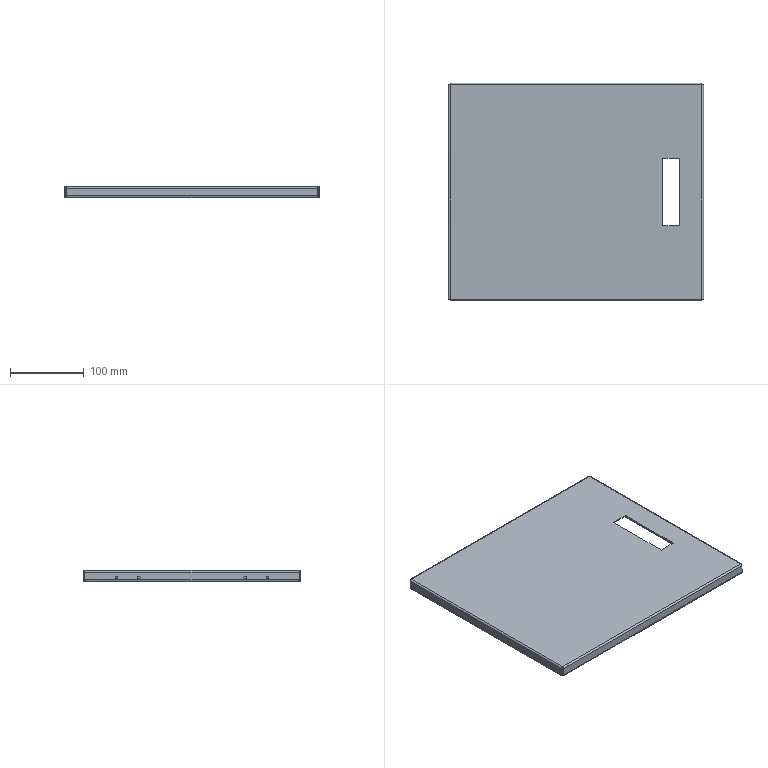Part | SolidWorks | features HoleWzd 3, ICE 3, EdgeFlange 2, Cut 1, FlatPattern 1, SMBaseFlange 1, SheetMetal 1, SolidToSheetMetal 1 | 1 solid | 82 faces | box 346 x 295 x 15 mm | volume 206058 mm3 | plane 42 | cylinder 24 | spline 16 | commonest cylinder face diameters 1.473 x8 3.3 x8 4.473 x8